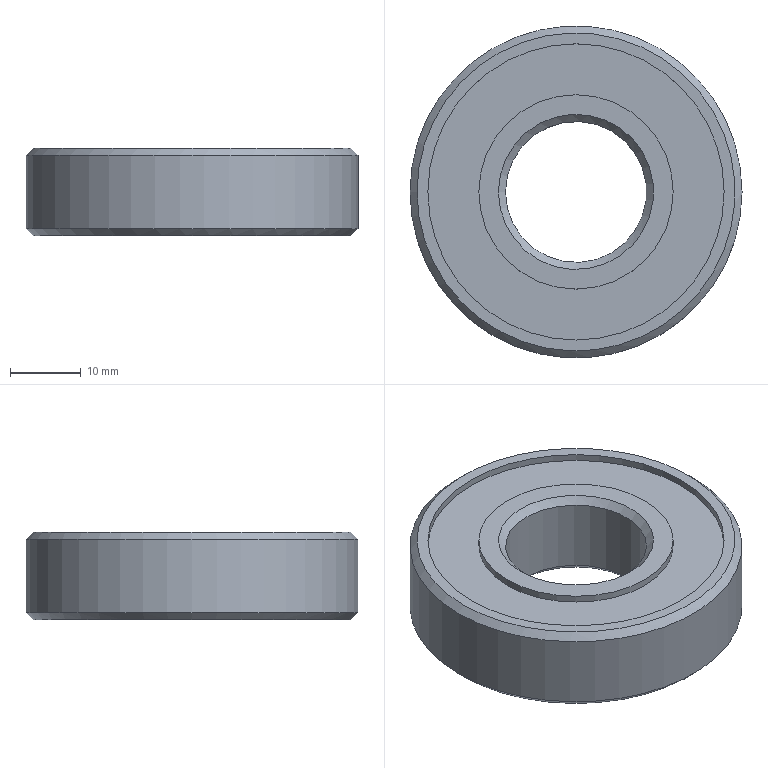Part | NX | features CHAMFER 4, DATUM_CSYS 4, EXTRUDE 3, SKETCH 3, DATUM_PLANE 1 | 1 solid | 16 faces | box 47.08 x 47.08 x 12.42 mm | volume 15931 mm3 | plane 6 | cylinder 6 | cone 4 | commonest cylinder face diameters 27.56 x2 42 x2 20 x1 47.08 x1
STEP:
#1=CARTESIAN_POINT('',(-11.,0.,0.));
#2=VERTEX_POINT('',#1);
#3=CARTESIAN_POINT('',(0.,0.,0.));
#4=DIRECTION('',(0.,0.,-1.));
#5=DIRECTION('',(-1.,0.,0.));
#6=AXIS2_PLACEMENT_3D('',#3,#4,#5);
#7=CIRCLE('',#6,11.);
#8=EDGE_CURVE('',#2,#2,#7,.F.);
#9=ORIENTED_EDGE('',*,*,#8,.T.);
#10=EDGE_LOOP('',(#9));
#11=FACE_BOUND('',#10,.T.);
#12=CARTESIAN_POINT('',(13.78,0.,0.));
#13=VERTEX_POINT('',#12);
#14=CARTESIAN_POINT('',(0.,0.,0.));
#15=DIRECTION('',(0.,0.,1.));
#16=DIRECTION('',(1.,0.,0.));
#17=AXIS2_PLACEMENT_3D('',#14,#15,#16);
#18=CIRCLE('',#17,13.78);
#19=EDGE_CURVE('',#13,#13,#18,.T.);
#20=ORIENTED_EDGE('',*,*,#19,.F.);
#21=EDGE_LOOP('',(#20));
#22=FACE_BOUND('',#21,.T.);
#23=CARTESIAN_POINT('',(0.,0.,0.));
#24=DIRECTION('',(0.,0.,-1.));
#25=DIRECTION('',(-1.,0.,0.));
#26=AXIS2_PLACEMENT_3D('',#23,#24,#25);
#27=PLANE('',#26);
#28=ADVANCED_FACE('',(#11,#22),#27,.T.);
#29=CARTESIAN_POINT('',(-11.,0.,12.42));
#30=VERTEX_POINT('',#29);
#31=CARTESIAN_POINT('',(0.,0.,12.42));
#32=DIRECTION('',(0.,0.,-1.));
#33=DIRECTION('',(-1.,0.,0.));
#34=AXIS2_PLACEMENT_3D('',#31,#32,#33);
#35=CIRCLE('',#34,11.);
#36=EDGE_CURVE('',#30,#30,#35,.T.);
#37=ORIENTED_EDGE('',*,*,#36,.T.);
#38=EDGE_LOOP('',(#37));
#39=FACE_BOUND('',#38,.T.);
#40=CARTESIAN_POINT('',(13.78,0.,12.42));
#41=VERTEX_POINT('',#40);
#42=CARTESIAN_POINT('',(0.,0.,12.42));
#43=DIRECTION('',(0.,0.,-1.));
#44=DIRECTION('',(1.,0.,0.));
#45=AXIS2_PLACEMENT_3D('',#42,#43,#44);
#46=CIRCLE('',#45,13.78);
#47=EDGE_CURVE('',#41,#41,#46,.T.);
#48=ORIENTED_EDGE('',*,*,#47,.F.);
#49=EDGE_LOOP('',(#48));
#50=FACE_BOUND('',#49,.T.);
#51=CARTESIAN_POINT('',(0.,0.,12.42));
#52=DIRECTION('',(0.,0.,-1.));
#53=DIRECTION('',(-1.,0.,0.));
#54=AXIS2_PLACEMENT_3D('',#51,#52,#53);
#55=PLANE('',#54);
#56=ADVANCED_FACE('',(#39,#50),#55,.F.);
#57=CARTESIAN_POINT('',(-23.54,0.,11.42));
#58=VERTEX_POINT('',#57);
#59=CARTESIAN_POINT('',(0.,0.,11.42));
#60=DIRECTION('',(0.,0.,-1.));
#61=DIRECTION('',(-1.,0.,0.));
#62=AXIS2_PLACEMENT_3D('',#59,#60,#61);
#63=CIRCLE('',#62,23.54);
#64=EDGE_CURVE('',#58,#58,#63,.T.);
#65=ORIENTED_EDGE('',*,*,#64,.T.);
#66=EDGE_LOOP('',(#65));
#67=FACE_BOUND('',#66,.T.);
#68=CARTESIAN_POINT('',(-23.54,0.,1.));
#69=VERTEX_POINT('',#68);
#70=CARTESIAN_POINT('',(0.,0.,1.));
#71=DIRECTION('',(0.,0.,-1.));
#72=DIRECTION('',(-1.,0.,0.));
#73=AXIS2_PLACEMENT_3D('',#70,#71,#72);
#74=CIRCLE('',#73,23.54);
#75=EDGE_CURVE('',#69,#69,#74,.F.);
#76=ORIENTED_EDGE('',*,*,#75,.T.);
#77=EDGE_LOOP('',(#76));
#78=FACE_BOUND('',#77,.T.);
#79=CARTESIAN_POINT('',(0.,0.,12.42));
#80=DIRECTION('',(0.,0.,-1.));
#81=DIRECTION('',(-1.,0.,0.));
#82=AXIS2_PLACEMENT_3D('',#79,#80,#81);
#83=CYLINDRICAL_SURFACE('',#82,23.54);
#84=ADVANCED_FACE('',(#67,#78),#83,.T.);
#85=CARTESIAN_POINT('',(-10.,0.,11.42));
#86=VERTEX_POINT('',#85);
#87=CARTESIAN_POINT('',(0.,0.,11.42));
#88=DIRECTION('',(0.,0.,-1.));
#89=DIRECTION('',(-1.,0.,0.));
#90=AXIS2_PLACEMENT_3D('',#87,#88,#89);
#91=CIRCLE('',#90,10.);
#92=EDGE_CURVE('',#86,#86,#91,.F.);
#93=ORIENTED_EDGE('',*,*,#92,.T.);
#94=EDGE_LOOP('',(#93));
#95=FACE_BOUND('',#94,.T.);
#96=CARTESIAN_POINT('',(-10.,0.,1.));
#97=VERTEX_POINT('',#96);
#98=CARTESIAN_POINT('',(0.,0.,1.));
#99=DIRECTION('',(0.,0.,-1.));
#100=DIRECTION('',(-1.,0.,0.));
#101=AXIS2_PLACEMENT_3D('',#98,#99,#100);
#102=CIRCLE('',#101,10.);
#103=EDGE_CURVE('',#97,#97,#102,.T.);
#104=ORIENTED_EDGE('',*,*,#103,.T.);
#105=EDGE_LOOP('',(#104));
#106=FACE_BOUND('',#105,.T.);
#107=CARTESIAN_POINT('',(0.,0.,12.42));
#108=DIRECTION('',(0.,0.,-1.));
#109=DIRECTION('',(-1.,0.,0.));
#110=AXIS2_PLACEMENT_3D('',#107,#108,#109);
#111=CYLINDRICAL_SURFACE('',#110,10.);
#112=ADVANCED_FACE('',(#95,#106),#111,.F.);
#113=CARTESIAN_POINT('',(-22.54,0.,12.42));
#114=VERTEX_POINT('',#113);
#115=CARTESIAN_POINT('',(0.,0.,12.42));
#116=DIRECTION('',(0.,0.,-1.));
#117=DIRECTION('',(-1.,0.,0.));
#118=AXIS2_PLACEMENT_3D('',#115,#116,#117);
#119=CIRCLE('',#118,22.54);
#120=EDGE_CURVE('',#114,#114,#119,.F.);
#121=ORIENTED_EDGE('',*,*,#120,.T.);
#122=EDGE_LOOP('',(#121));
#123=FACE_BOUND('',#122,.T.);
#124=CARTESIAN_POINT('',(21.,0.,12.42));
#125=VERTEX_POINT('',#124);
#126=CARTESIAN_POINT('',(0.,0.,12.42));
#127=DIRECTION('',(0.,0.,-1.));
#128=DIRECTION('',(1.,0.,0.));
#129=AXIS2_PLACEMENT_3D('',#126,#127,#128);
#130=CIRCLE('',#129,21.);
#131=EDGE_CURVE('',#125,#125,#130,.T.);
#132=ORIENTED_EDGE('',*,*,#131,.T.);
#133=EDGE_LOOP('',(#132));
#134=FACE_BOUND('',#133,.T.);
#135=CARTESIAN_POINT('',(0.,0.,12.42));
#136=DIRECTION('',(0.,0.,-1.));
#137=DIRECTION('',(-1.,0.,0.));
#138=AXIS2_PLACEMENT_3D('',#135,#136,#137);
#139=PLANE('',#138);
#140=ADVANCED_FACE('',(#123,#134),#139,.F.);
#141=CARTESIAN_POINT('',(-22.54,0.,0.));
#142=VERTEX_POINT('',#141);
#143=CARTESIAN_POINT('',(0.,0.,0.));
#144=DIRECTION('',(0.,0.,-1.));
#145=DIRECTION('',(-1.,0.,0.));
#146=AXIS2_PLACEMENT_3D('',#143,#144,#145);
#147=CIRCLE('',#146,22.54);
#148=EDGE_CURVE('',#142,#142,#147,.T.);
#149=ORIENTED_EDGE('',*,*,#148,.T.);
#150=EDGE_LOOP('',(#149));
#151=FACE_BOUND('',#150,.T.);
#152=CARTESIAN_POINT('',(21.,0.,0.));
#153=VERTEX_POINT('',#152);
#154=CARTESIAN_POINT('',(0.,0.,0.));
#155=DIRECTION('',(0.,0.,1.));
#156=DIRECTION('',(1.,0.,0.));
#157=AXIS2_PLACEMENT_3D('',#154,#155,#156);
#158=CIRCLE('',#157,21.);
#159=EDGE_CURVE('',#153,#153,#158,.T.);
#160=ORIENTED_EDGE('',*,*,#159,.T.);
#161=EDGE_LOOP('',(#160));
#162=FACE_BOUND('',#161,.T.);
#163=CARTESIAN_POINT('',(0.,0.,0.));
#164=DIRECTION('',(0.,0.,-1.));
#165=DIRECTION('',(-1.,0.,0.));
#166=AXIS2_PLACEMENT_3D('',#163,#164,#165);
#167=PLANE('',#166);
#168=ADVANCED_FACE('',(#151,#162),#167,.T.);
#169=CARTESIAN_POINT('',(21.,0.,11.42));
#170=VERTEX_POINT('',#169);
#171=CARTESIAN_POINT('',(0.,0.,11.42));
#172=DIRECTION('',(0.,0.,-1.));
#173=DIRECTION('',(1.,0.,0.));
#174=AXIS2_PLACEMENT_3D('',#171,#172,#173);
#175=CIRCLE('',#174,21.);
#176=EDGE_CURVE('',#170,#170,#175,.F.);
#177=ORIENTED_EDGE('',*,*,#176,.F.);
#178=EDGE_LOOP('',(#177));
#179=FACE_BOUND('',#178,.T.);
#180=ORIENTED_EDGE('',*,*,#131,.F.);
#181=EDGE_LOOP('',(#180));
#182=FACE_BOUND('',#181,.T.);
#183=CARTESIAN_POINT('',(0.,0.,11.42));
#184=DIRECTION('',(0.,0.,1.));
#185=DIRECTION('',(1.,0.,0.));
#186=AXIS2_PLACEMENT_3D('',#183,#184,#185);
#187=CYLINDRICAL_SURFACE('',#186,21.);
#188=ADVANCED_FACE('',(#179,#182),#187,.F.);
#189=CARTESIAN_POINT('',(13.78,0.,11.42));
#190=VERTEX_POINT('',#189);
#191=CARTESIAN_POINT('',(0.,0.,11.42));
#192=DIRECTION('',(0.,0.,-1.));
#193=DIRECTION('',(1.,0.,0.));
#194=AXIS2_PLACEMENT_3D('',#191,#192,#193);
#195=CIRCLE('',#194,13.78);
#196=EDGE_CURVE('',#190,#190,#195,.F.);
#197=ORIENTED_EDGE('',*,*,#196,.T.);
#198=EDGE_LOOP('',(#197));
#199=FACE_BOUND('',#198,.T.);
#200=ORIENTED_EDGE('',*,*,#47,.T.);
#201=EDGE_LOOP('',(#200));
#202=FACE_BOUND('',#201,.T.);
#203=CARTESIAN_POINT('',(0.,0.,11.42));
#204=DIRECTION('',(0.,0.,1.));
#205=DIRECTION('',(1.,0.,0.));
#206=AXIS2_PLACEMENT_3D('',#203,#204,#205);
#207=CYLINDRICAL_SURFACE('',#206,13.78);
#208=ADVANCED_FACE('',(#199,#202),#207,.T.);
#209=ORIENTED_EDGE('',*,*,#176,.T.);
#210=EDGE_LOOP('',(#209));
#211=FACE_BOUND('',#210,.T.);
#212=ORIENTED_EDGE('',*,*,#196,.F.);
#213=EDGE_LOOP('',(#212));
#214=FACE_BOUND('',#213,.T.);
#215=CARTESIAN_POINT('',(0.,0.,11.42));
#216=DIRECTION('',(0.,0.,-1.));
#217=DIRECTION('',(-1.,0.,0.));
#218=AXIS2_PLACEMENT_3D('',#215,#216,#217);
#219=PLANE('',#218);
#220=ADVANCED_FACE('',(#211,#214),#219,.F.);
#221=CARTESIAN_POINT('',(21.,0.,1.));
#222=VERTEX_POINT('',#221);
#223=CARTESIAN_POINT('',(0.,0.,1.));
#224=DIRECTION('',(0.,0.,1.));
#225=DIRECTION('',(1.,0.,0.));
#226=AXIS2_PLACEMENT_3D('',#223,#224,#225);
#227=CIRCLE('',#226,21.);
#228=EDGE_CURVE('',#222,#222,#227,.F.);
#229=ORIENTED_EDGE('',*,*,#228,.F.);
#230=EDGE_LOOP('',(#229));
#231=FACE_BOUND('',#230,.T.);
#232=ORIENTED_EDGE('',*,*,#159,.F.);
#233=EDGE_LOOP('',(#232));
#234=FACE_BOUND('',#233,.T.);
#235=CARTESIAN_POINT('',(0.,0.,1.));
#236=DIRECTION('',(0.,0.,-1.));
#237=DIRECTION('',(-1.,0.,0.));
#238=AXIS2_PLACEMENT_3D('',#235,#236,#237);
#239=CYLINDRICAL_SURFACE('',#238,21.);
#240=ADVANCED_FACE('',(#231,#234),#239,.F.);
#241=CARTESIAN_POINT('',(13.78,0.,1.));
#242=VERTEX_POINT('',#241);
#243=CARTESIAN_POINT('',(0.,0.,1.));
#244=DIRECTION('',(0.,0.,1.));
#245=DIRECTION('',(1.,0.,0.));
#246=AXIS2_PLACEMENT_3D('',#243,#244,#245);
#247=CIRCLE('',#246,13.78);
#248=EDGE_CURVE('',#242,#242,#247,.F.);
#249=ORIENTED_EDGE('',*,*,#248,.T.);
#250=EDGE_LOOP('',(#249));
#251=FACE_BOUND('',#250,.T.);
#252=ORIENTED_EDGE('',*,*,#19,.T.);
#253=EDGE_LOOP('',(#252));
#254=FACE_BOUND('',#253,.T.);
#255=CARTESIAN_POINT('',(0.,0.,1.));
#256=DIRECTION('',(0.,0.,-1.));
#257=DIRECTION('',(-1.,0.,0.));
#258=AXIS2_PLACEMENT_3D('',#255,#256,#257);
#259=CYLINDRICAL_SURFACE('',#258,13.78);
#260=ADVANCED_FACE('',(#251,#254),#259,.T.);
#261=ORIENTED_EDGE('',*,*,#228,.T.);
#262=EDGE_LOOP('',(#261));
#263=FACE_BOUND('',#262,.T.);
#264=ORIENTED_EDGE('',*,*,#248,.F.);
#265=EDGE_LOOP('',(#264));
#266=FACE_BOUND('',#265,.T.);
#267=CARTESIAN_POINT('',(0.,0.,1.));
#268=DIRECTION('',(0.,0.,1.));
#269=DIRECTION('',(1.,0.,0.));
#270=AXIS2_PLACEMENT_3D('',#267,#268,#269);
#271=PLANE('',#270);
#272=ADVANCED_FACE('',(#263,#266),#271,.F.);
#273=ORIENTED_EDGE('',*,*,#75,.F.);
#274=EDGE_LOOP('',(#273));
#275=FACE_BOUND('',#274,.T.);
#276=ORIENTED_EDGE('',*,*,#148,.F.);
#277=EDGE_LOOP('',(#276));
#278=FACE_BOUND('',#277,.T.);
#279=CARTESIAN_POINT('',(0.,0.,0.));
#280=DIRECTION('',(0.,0.,1.));
#281=DIRECTION('',(1.,0.,0.));
#282=AXIS2_PLACEMENT_3D('',#279,#280,#281);
#283=CONICAL_SURFACE('',#282,22.54,0.7854);
#284=ADVANCED_FACE('',(#275,#278),#283,.T.);
#285=ORIENTED_EDGE('',*,*,#120,.F.);
#286=EDGE_LOOP('',(#285));
#287=FACE_BOUND('',#286,.T.);
#288=ORIENTED_EDGE('',*,*,#64,.F.);
#289=EDGE_LOOP('',(#288));
#290=FACE_BOUND('',#289,.T.);
#291=CARTESIAN_POINT('',(0.,0.,11.42));
#292=DIRECTION('',(0.,0.,-1.));
#293=DIRECTION('',(-1.,0.,0.));
#294=AXIS2_PLACEMENT_3D('',#291,#292,#293);
#295=CONICAL_SURFACE('',#294,23.54,0.7854);
#296=ADVANCED_FACE('',(#287,#290),#295,.T.);
#297=ORIENTED_EDGE('',*,*,#8,.F.);
#298=EDGE_LOOP('',(#297));
#299=FACE_BOUND('',#298,.T.);
#300=ORIENTED_EDGE('',*,*,#103,.F.);
#301=EDGE_LOOP('',(#300));
#302=FACE_BOUND('',#301,.T.);
#303=CARTESIAN_POINT('',(0.,0.,1.));
#304=DIRECTION('',(0.,0.,-1.));
#305=DIRECTION('',(-1.,0.,0.));
#306=AXIS2_PLACEMENT_3D('',#303,#304,#305);
#307=CONICAL_SURFACE('',#306,10.,0.7854);
#308=ADVANCED_FACE('',(#299,#302),#307,.F.);
#309=ORIENTED_EDGE('',*,*,#92,.F.);
#310=EDGE_LOOP('',(#309));
#311=FACE_BOUND('',#310,.T.);
#312=ORIENTED_EDGE('',*,*,#36,.F.);
#313=EDGE_LOOP('',(#312));
#314=FACE_BOUND('',#313,.T.);
#315=CARTESIAN_POINT('',(0.,0.,12.42));
#316=DIRECTION('',(0.,0.,1.));
#317=DIRECTION('',(1.,0.,0.));
#318=AXIS2_PLACEMENT_3D('',#315,#316,#317);
#319=CONICAL_SURFACE('',#318,11.,0.7854);
#320=ADVANCED_FACE('',(#311,#314),#319,.F.);
#321=CLOSED_SHELL('',(#28,#56,#84,#112,#140,#168,#188,#208,#220,#240,#260,#272,#284,#296,#308,#320));
#322=MANIFOLD_SOLID_BREP('',#321);
#323=(LENGTH_UNIT()NAMED_UNIT(*)SI_UNIT(.MILLI.,.METRE.));
#324=UNCERTAINTY_MEASURE_WITH_UNIT(LENGTH_MEASURE(0.00001),#323,'','');
#325=(NAMED_UNIT(*)PLANE_ANGLE_UNIT()SI_UNIT($,.RADIAN.));
#326=(NAMED_UNIT(*)SI_UNIT($,.STERADIAN.)SOLID_ANGLE_UNIT());
#327=(GEOMETRIC_REPRESENTATION_CONTEXT(3)GLOBAL_UNCERTAINTY_ASSIGNED_CONTEXT((#324))GLOBAL_UNIT_ASSIGNED_CONTEXT((#323,#325,#326))REPRESENTATION_CONTEXT('',''));
#328=ADVANCED_BREP_SHAPE_REPRESENTATION('',(#322),#327);